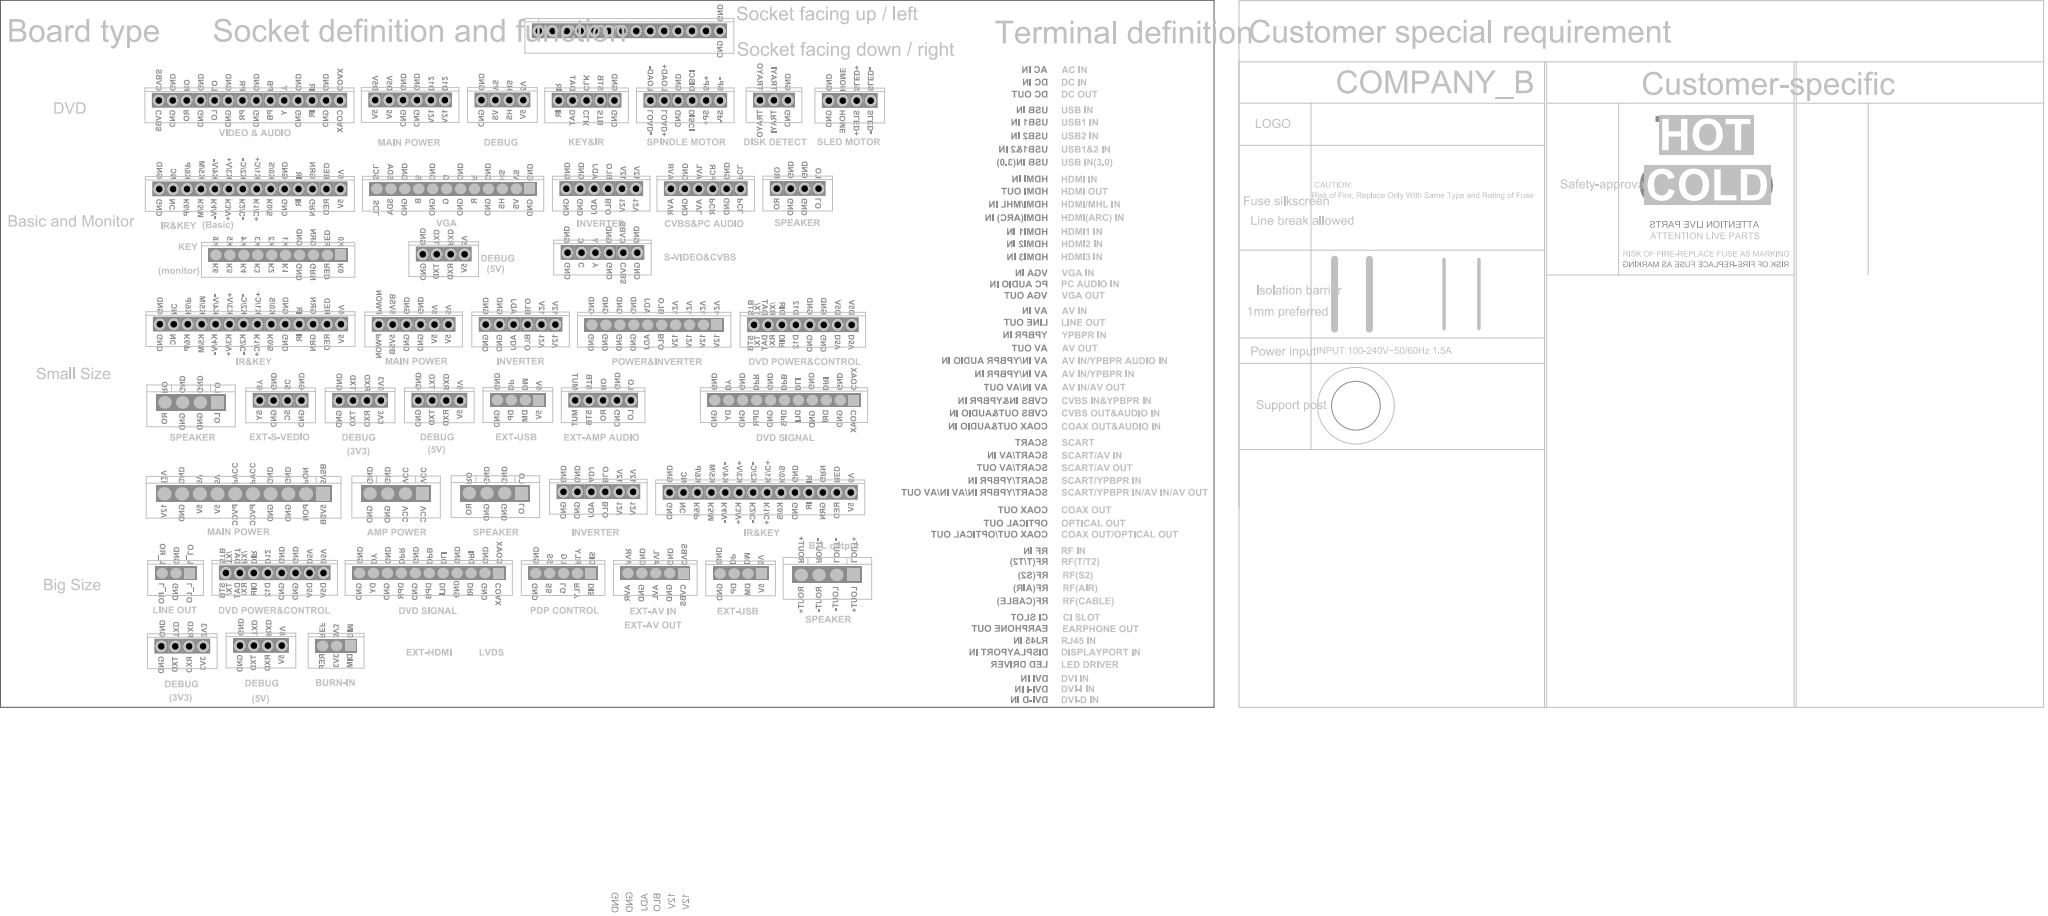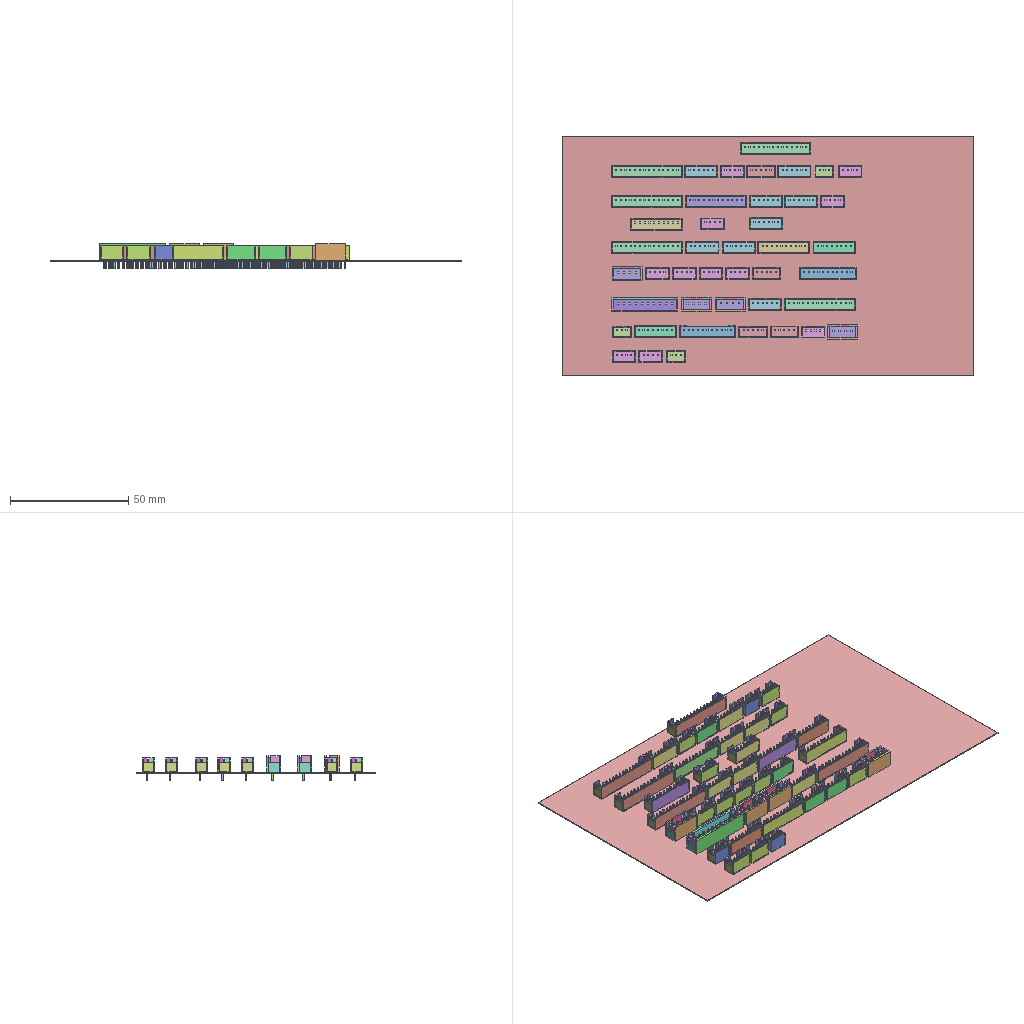Circuit board layout | Altium Designer | box 174.2 x 101.5 x 10.5 mm
Part placement:
Designator,Comment,Layer,Footprint,Center-X(mm),Center-Y(mm),Rotation
SPEAKER 0,4PIN-2.54-D-H-G,TopLayer,SIP4/2.54DA,118.684,19.004,360
IR&KEY3,14PIN-2.0-D-H-G,TopLayer,SIP10/2.0DA,39.857,64.925,360
EXT-S-VEDIO1,4PIN-2.0-D-H-G,TopLayer,SIP5/2.0DA,86.493,44.061,360
EXT-USB1,NC/4PIN-2.0-D-H-G,TopLayer,SIP4/2.0DA,74.259,44.09,360
SPEAKER ,4PIN-2.54-D-H-G,TopLayer,SIP4/2.0DA,114.417,74.449,360
DEBUG,4PIN-2.0-D-H-blue-G,TopLayer,SIP4/2.0DA,51.613,44.041,360
AMP POWER,4PIN-2.54-D-H-red-G,TopLayer,SIP4/2.54DA,56.785,30.688,360
DEBUG,4PIN-2.0-D-H-G,TopLayer,SIP4/2.0DA,62.98,44.041,360
VGA,NC/14PIN-2.0-D-H-G,TopLayer,SIP12/2.0DA,64.968,74.424,360
AV&PC AUDIO ,NC/6PIN-2.0-D-H-G,TopLayer,SIP6/2.0DA,101.225,74.424,360
S-VIDEO&CVBS ,NC/6PIN-2.0-D-H,TopLayer,SIP6/2.0DA,86.398,65.257,0
SPINDLE MOTOR,6PIN-2.0-L-H-G,TopLayer,SIP6/2.0DA,98.285,87.104,360
VIDEO AND AUDIO ,14PIN-2.0-L-H-G,TopLayer,SIP14/2.0DA,35.737,87.11,360
MAIN POWER,6PIN-2.0-L-H-G,TopLayer,SIP6/2.0DA,58.794,87.155,360
SLED MOTOR,4PIN-2.0-L-H-G,TopLayer,SIP4/2.0DA,121.893,87.079,360
DISK DETECT,3PIN-2.0-L-H-G,TopLayer,SIP3/2.0DA,111.013,87.13,360
KEY&IR,5PIN-2.0-L-H-G,TopLayer,SIP5/2.0DA,84.118,87.104,360
HS&VS,4PIN-2.0-L-H-G,TopLayer,SIP4/2.0DA,72.04,87.155,360
POWER&INVERTER,NC/6PIN-2.0-D-H-G,TopLayer,SIP10/2.0DA,93.828,54.892,360
POWER,NC/4PIN-2.0-D-H-G,TopLayer,SIP6/2.0DA,59.299,54.938,360
EXT-S-VEDIO,4PIN-2.0-D-H-G,TopLayer,SIP4/2.0DA,40.209,44.044,360
MAIN POWER,10PIN-2.54-D-H-G,TopLayer,SIP10/2.54DA,34.896,30.644,360
INVERTER,6PIN-2.0-D-H-G,TopLayer,SIP6/2.0DA,85.809,30.928,360
PDP,NC/5PIN-2.0-D-H-G,TopLayer,SIP5/2.0DA,80.751,19.247,360
IR&KEY,14PIN-2.0-D-H-G,TopLayer,SIP14/2.0DA,109.037,30.834,360
EXT-USB,NC/4PIN-2.0-D-H-G,TopLayer,SIP4/2.0DA,106.229,19.201,360
LINE OUT,3PIN-2.0-D-H-G,TopLayer,SIP3/2.0DA,25.137,19.253,360
DVD SIGNAL,11PIN-2.0-D-H-G,TopLayer,SIP11/2.0DA,61.47,19.269,360
DVD POWER&CONTROL,6PIN-2.0-D-H-G,TopLayer,SIP8/2.0DA,39.367,19.285,360
SPEAKER ,4PIN-2.54-D-H-G,TopLayer,SIP4/2.54DA,71.034,30.738,360
SPEAKER 1,4PIN-2.54-D-H-G,TopLayer,SIP4/2.54DA,27.358,43.764,360
DEBUG_1,4PIN-2.0-D-H-G,TopLayer,SIP4/2.0DA,37.387,8.853,360
DEBUG_1,4PIN-2.0-D-H-blue-G,TopLayer,SIP4/2.0DA,26.095,8.752,360
IR&KEY1,14PIN-2.0-D-H-G,TopLayer,SIP14/2.0DA,35.884,54.983,360
INVERTER1,6PIN-2.0-D-H-G,TopLayer,SIP6/2.0DA,74.647,54.938,360
DVD POWER&CONTROL_1,6PIN-2.0-D-H-G,TopLayer,SIP8/2.0DA,115.162,54.892,360
DVD SIGNAL_1,11PIN-2.0-D-H-G,TopLayer,SIP11/2.0DA,112.455,44.081,360
IR&KEY2,14PIN-2.0-D-H-G,TopLayer,SIP14/2.0DA,35.793,74.389,360
INVERTER2,6PIN-2.0-D-H-G,TopLayer,SIP6/2.0DA,86.222,74.433,360
DEBUG_2,4PIN-2.0-D-H-G,TopLayer,SIP4/2.0DA,63.62,65.027,360
CN17,5PIN-2.0-D-H-G,TopLayer,SIP5/2.0DA,93.983,19.258,360
VIDEO AND AUDIO 1,14PIN-2.0-L-H-G,TopLayer,SIP14/2.0DA,90.262,97.083,360
LINE OUT1,3PIN-2.0-D-H-G,TopLayer,SIP3/2.0DA,48.175,8.813,360